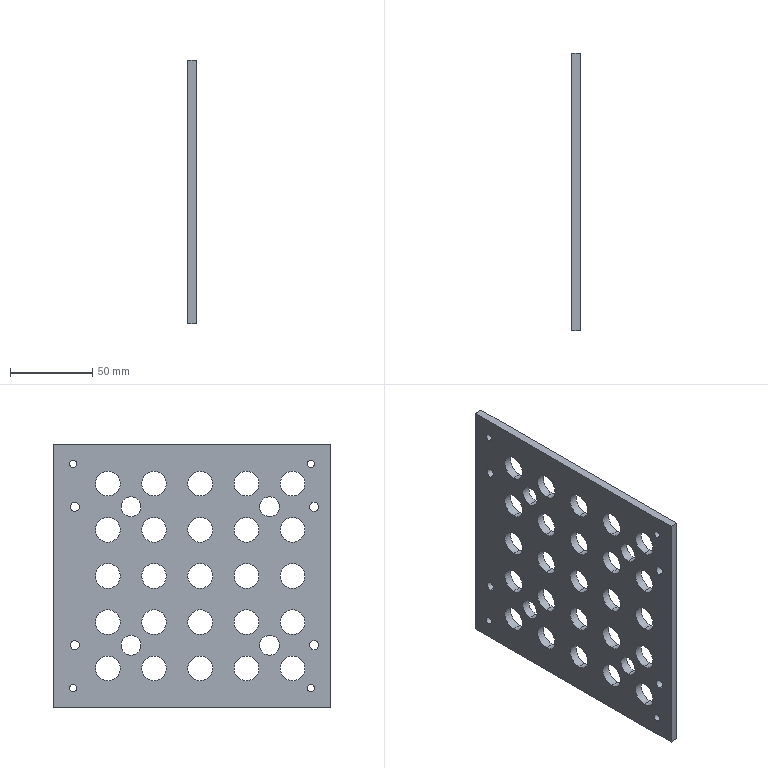Part | STEP file | 03-11 Suction cup fixing plate | 1 solid | 80 faces | box 5 x 168 x 160 mm | volume 109255 mm3 | cylinder 74 | plane 6 | commonest cylinder face diameters 15 x50 4.5 x8 5.5 x8 12 x8